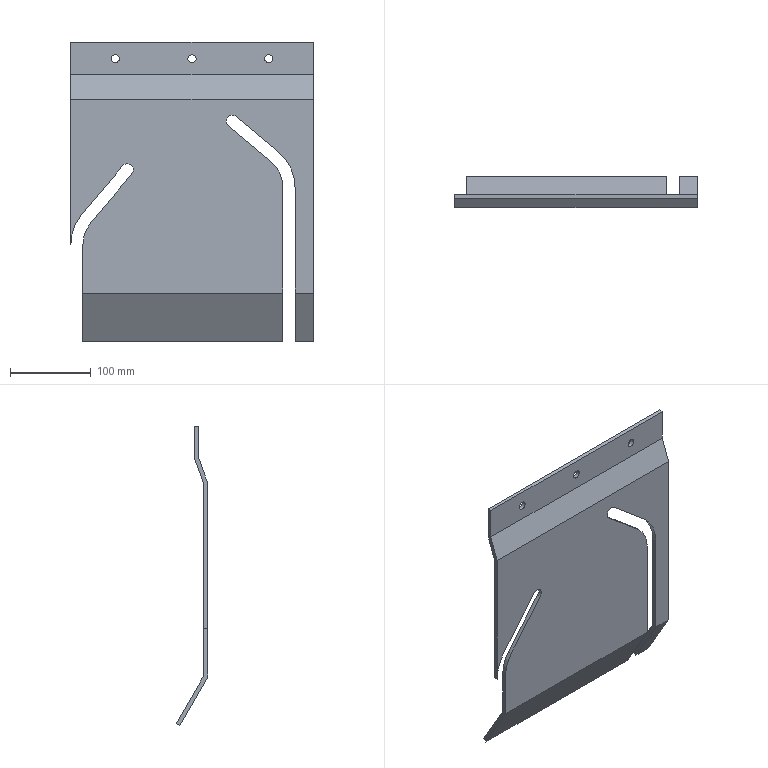Part | STEP file | gudingzhezhiban2 | 1 solid | 31 faces | box 300 x 38.971 x 370 mm | volume 526356 mm3 | plane 22 | cylinder 9 | commonest cylinder face diameters 10 x3 15 x2 85 x2 115 x2